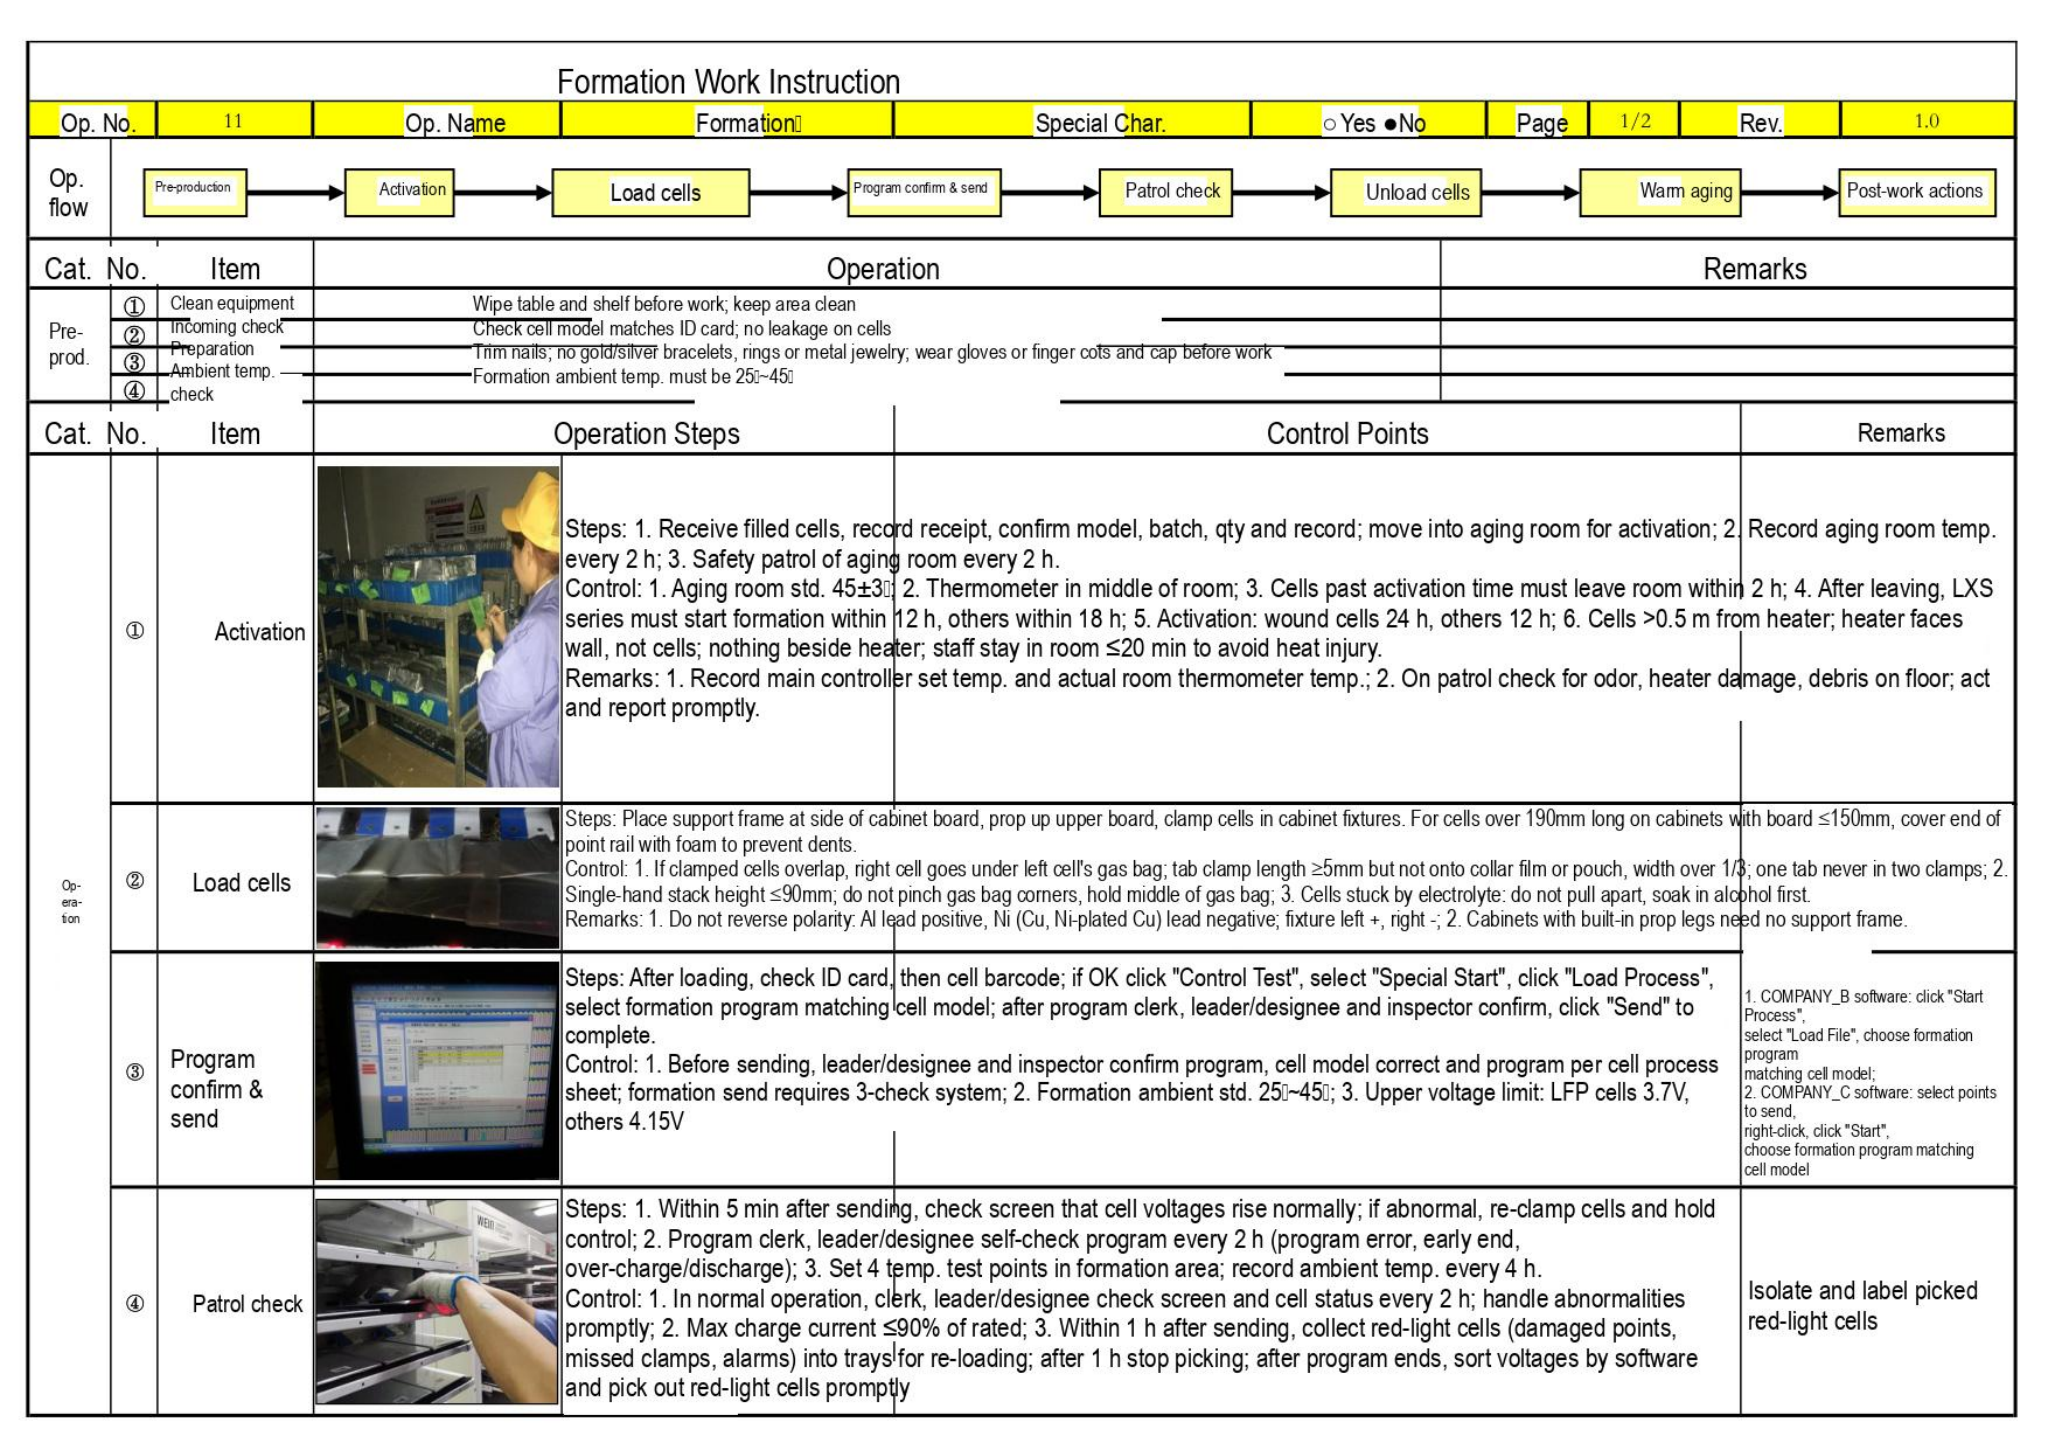Formation Work Instruction

| Op. No. | 11 | Op. Name | Formation | Special Char. | ○ Yes ●No | Page | 1/2 | Rev. | 1.0 |
|---|---|---|---|---|---|---|---|---|---|

Op. flow: Pre-production → Activation → Load cells → Program confirm & send → Patrol check → Unload cells → Warm aging → Post-work actions

| Cat. | No. | Item | Operation | Remarks |
|---|---|---|---|---|
| Pre-prod. | ① | Clean equipment | Wipe table and shelf before work; keep area clean | |
| | ② | Incoming check | Check cell model matches ID card; no leakage on cells | |
| | ③ | Preparation | Trim nails; no gold/silver bracelets, rings or metal jewelry; wear gloves or finger cots and cap before work | |
| | ④ | Ambient temp. check | Formation ambient temp. must be 25~45 | |

| Cat. | No. | Item | Operation Steps | Control Points | Remarks |
|---|---|---|---|---|---|
| Op-era-tion | ① | Activation | Steps: 1. Receive filled cells, record receipt, confirm model, batch, qty and record; move into aging room for activation; 2. Record aging room temp. every 2 h; 3. Safety patrol of aging room every 2 h.<br>Control: 1. Aging room std. 45±3; 2. Thermometer in middle of room; 3. Cells past activation time must leave room within 2 h; 4. After leaving, LXS series must start formation within 12 h, others within 18 h; 5. Activation: wound cells 24 h, others 12 h; 6. Cells >0.5 m from heater; heater faces wall, not cells; nothing beside heater; staff stay in room ≤20 min to avoid heat injury.<br>Remarks: 1. Record main controller set temp. and actual room thermometer temp.; 2. On patrol check for odor, heater damage, debris on floor; act and report promptly. | | |
| | ② | Load cells | Steps: Place support frame at side of cabinet board, prop up upper board, clamp cells in cabinet fixtures. For cells over 190mm long on cabinets with board ≤150mm, cover end of point rail with foam to prevent dents.<br>Control: 1. If clamped cells overlap, right cell goes under left cell's gas bag; tab clamp length ≥5mm but not onto collar film or pouch, width over 1/3; one tab never in two clamps; 2. Single-hand stack height ≤90mm; do not pinch gas bag corners, hold middle of gas bag; 3. Cells stuck by electrolyte: do not pull apart, soak in alcohol first.<br>Remarks: 1. Do not reverse polarity: Al lead positive, Ni (Cu, Ni-plated Cu) lead negative; fixture left +, right -; 2. Cabinets with built-in prop legs need no support frame. | | |
| | ③ | Program confirm & send | Steps: After loading, check ID card, then cell barcode; if OK click "Control Test", select "Special Start", click "Load Process", select formation program matching cell model; after program clerk, leader/designee and inspector confirm, click "Send" to complete.<br>Control: 1. Before sending, leader/designee and inspector confirm program, cell model correct and program per cell process sheet; formation send requires 3-check system; 2. Formation ambient std. 25~45; 3. Upper voltage limit: LFP cells 3.7V, others 4.15V | | 1. COMPANY_B software: click "Start Process", select "Load File", choose formation program matching cell model;<br>2. COMPANY_C software: select points to send, right-click, click "Start", choose formation program matching cell model |
| | ④ | Patrol check | Steps: 1. Within 5 min after sending, check screen that cell voltages rise normally; if abnormal, re-clamp cells and hold control; 2. Program clerk, leader/designee self-check program every 2 h (program error, early end, over-charge/discharge); 3. Set 4 temp. test points in formation area; record ambient temp. every 4 h.<br>Control: 1. In normal operation, clerk, leader/designee check screen and cell status every 2 h; handle abnormalities promptly; 2. Max charge current ≤90% of rated; 3. Within 1 h after sending, collect red-light cells (damaged points, missed clamps, alarms) into trays for re-loading; after 1 h stop picking; after program ends, sort voltages by software and pick out red-light cells promptly | | Isolate and label picked red-light cells |

WEIN
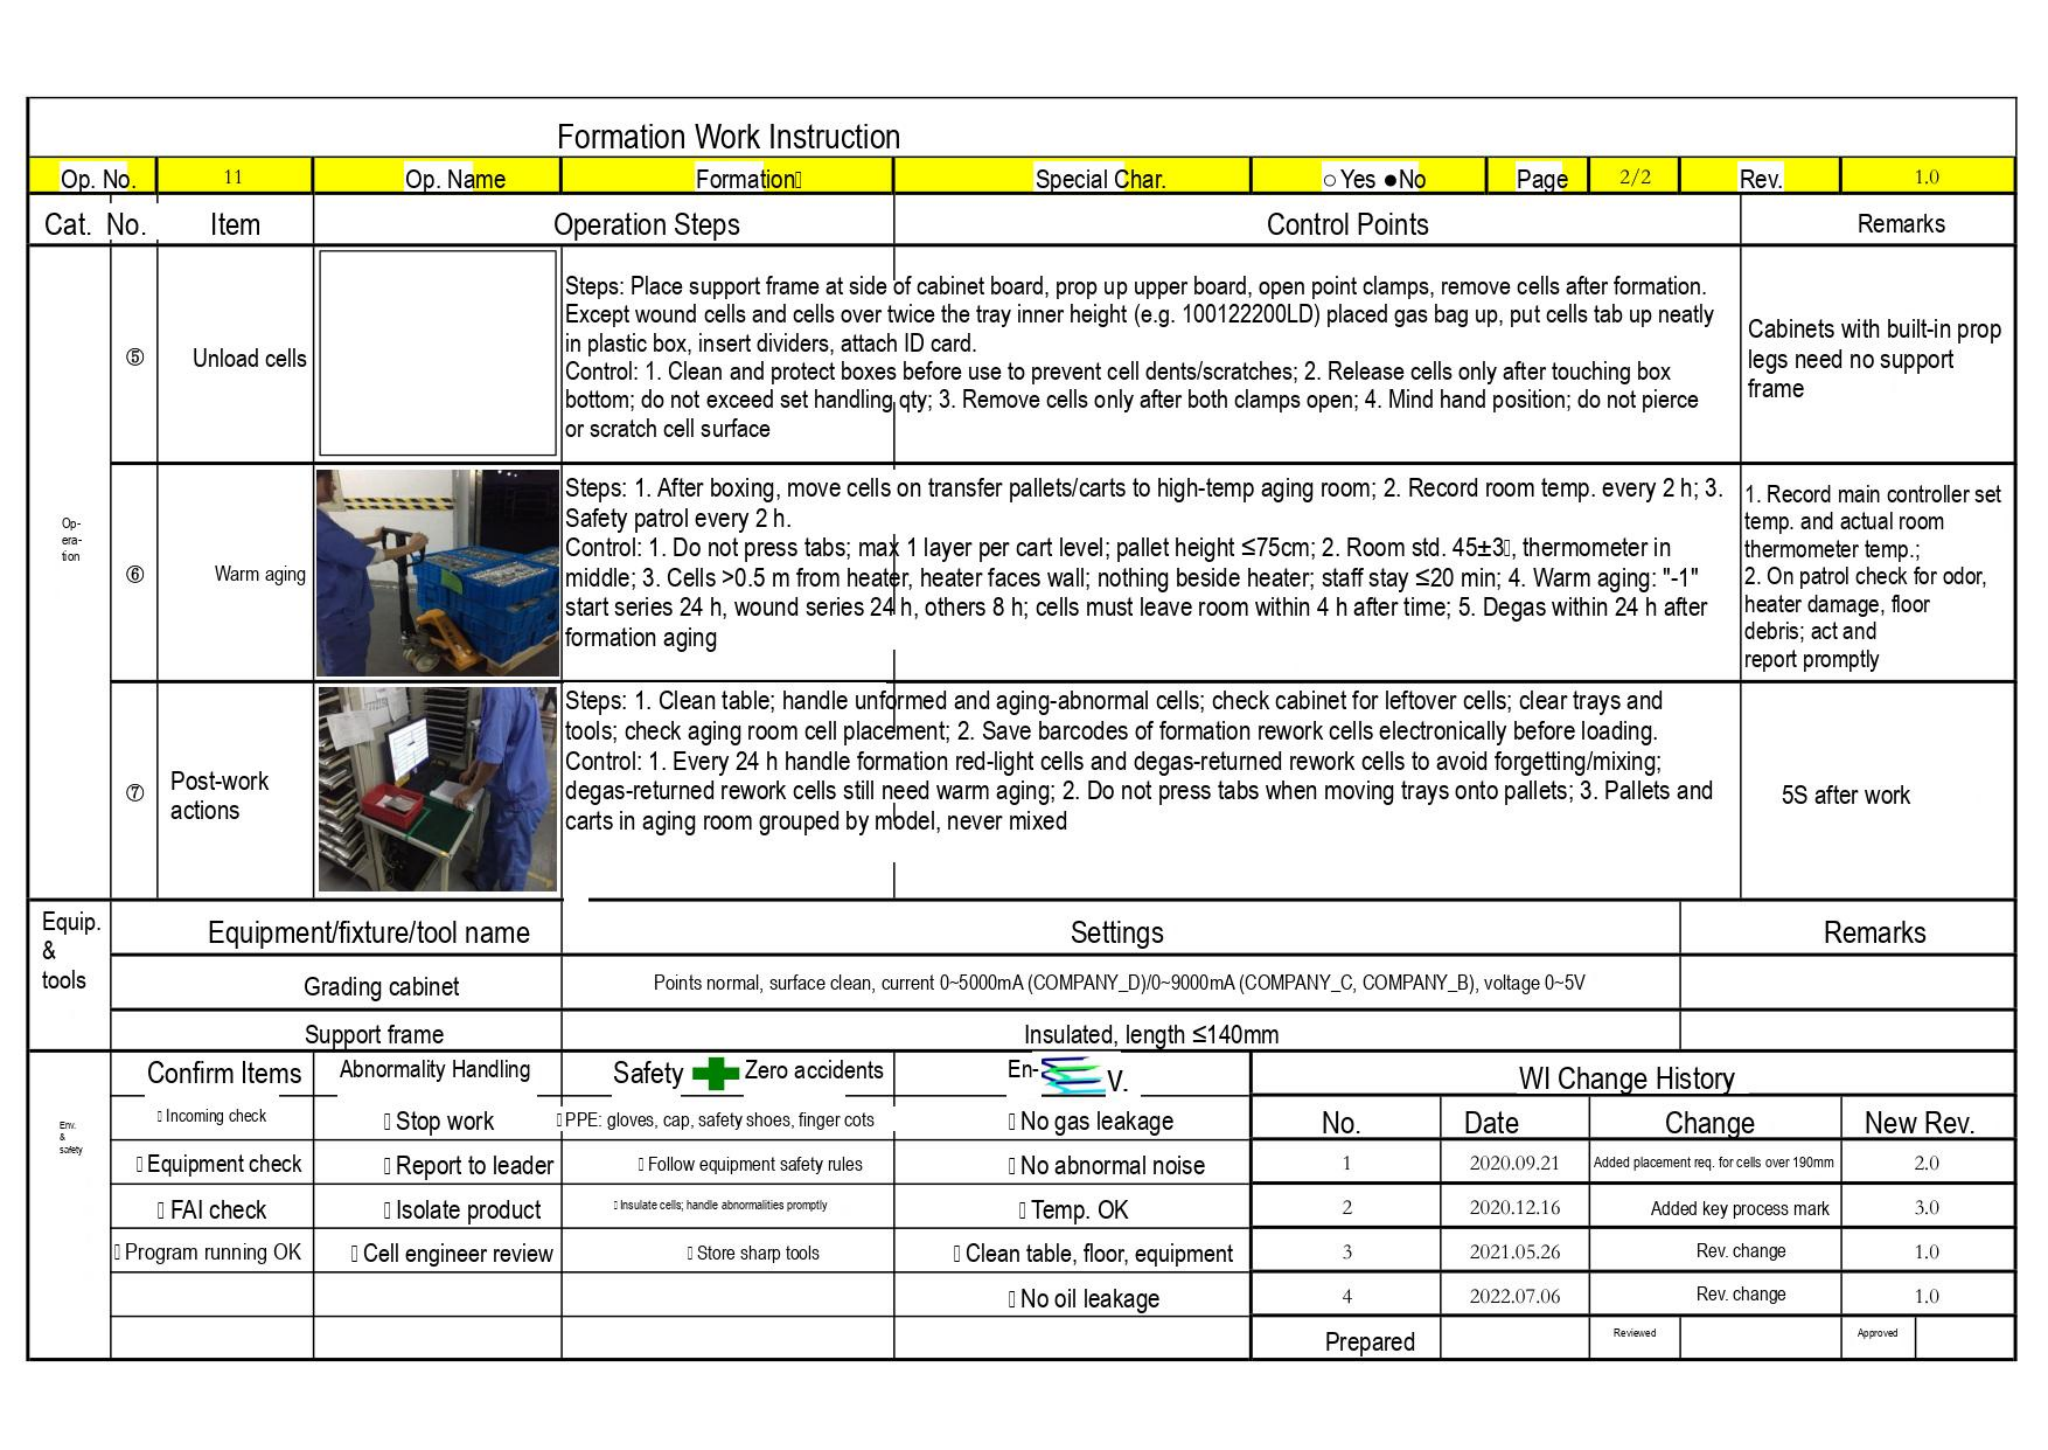Formation Work Instruction

| Op. No. | 11 | Op. Name | Formation | Special Char. | ○ Yes ●No | Page | 2/2 | Rev. | 1.0 |
|---|---|---|---|---|---|---|---|---|---|

| Cat. | No. | Item | Operation Steps | Control Points | Remarks |
|---|---|---|---|---|---|
| Op-era-tion | ⑤ | Unload cells | | Steps: Place support frame at side of cabinet board, prop up upper board, open point clamps, remove cells after formation. Except wound cells and cells over twice the tray inner height (e.g. 100122200LD) placed gas bag up, put cells tab up neatly in plastic box, insert dividers, attach ID card.<br>Control: 1. Clean and protect boxes before use to prevent cell dents/scratches; 2. Release cells only after touching box bottom; do not exceed set handling qty; 3. Remove cells only after both clamps open; 4. Mind hand position; do not pierce or scratch cell surface | Cabinets with built-in prop legs need no support frame |
| | ⑥ | Warm aging | | Steps: 1. After boxing, move cells on transfer pallets/carts to high-temp aging room; 2. Record room temp. every 2 h; 3. Safety patrol every 2 h.<br>Control: 1. Do not press tabs; max 1 layer per cart level; pallet height ≤75cm; 2. Room std. 45±3, thermometer in middle; 3. Cells >0.5 m from heater, heater faces wall; nothing beside heater; staff stay ≤20 min; 4. Warm aging: "-1" start series 24 h, wound series 24 h, others 8 h; cells must leave room within 4 h after time; 5. Degas within 24 h after formation aging | 1. Record main controller set temp. and actual room thermometer temp.;<br>2. On patrol check for odor, heater damage, floor debris; act and report promptly |
| | ⑦ | Post-work actions | | Steps: 1. Clean table; handle unformed and aging-abnormal cells; check cabinet for leftover cells; clear trays and tools; check aging room cell placement; 2. Save barcodes of formation rework cells electronically before loading.<br>Control: 1. Every 24 h handle formation red-light cells and degas-returned rework cells to avoid forgetting/mixing; degas-returned rework cells still need warm aging; 2. Do not press tabs when moving trays onto pallets; 3. Pallets and carts in aging room grouped by model, never mixed | 5S after work |

| Equip. & tools | Equipment/fixture/tool name | Settings | Remarks |
|---|---|---|---|
| | Grading cabinet | Points normal, surface clean, current 0~5000mA (COMPANY_D)/0~9000mA (COMPANY_C, COMPANY_B), voltage 0~5V | |
| | Support frame | Insulated, length ≤140mm | |

| Env. & safety | Confirm Items | Abnormality Handling | Safety Zero accidents | En-V. | WI Change History | | | |
|---|---|---|---|---|---|---|---|---|
| | Incoming check | Stop work | PPE: gloves, cap, safety shoes, finger cots | No gas leakage | No. | Date | Change | New Rev. |
| | Equipment check | Report to leader | Follow equipment safety rules | No abnormal noise | 1 | 2020.09.21 | Added placement req. for cells over 190mm | 2.0 |
| | FAI check | Isolate product | Insulate cells; handle abnormalities promptly | Temp. OK | 2 | 2020.12.16 | Added key process mark | 3.0 |
| | Program running OK | Cell engineer review | Store sharp tools | Clean table, floor, equipment | 3 | 2021.05.26 | Rev. change | 1.0 |
| | | | | No oil leakage | 4 | 2022.07.06 | Rev. change | 1.0 |
| | | | | | Prepared | | Reviewed | Approved |